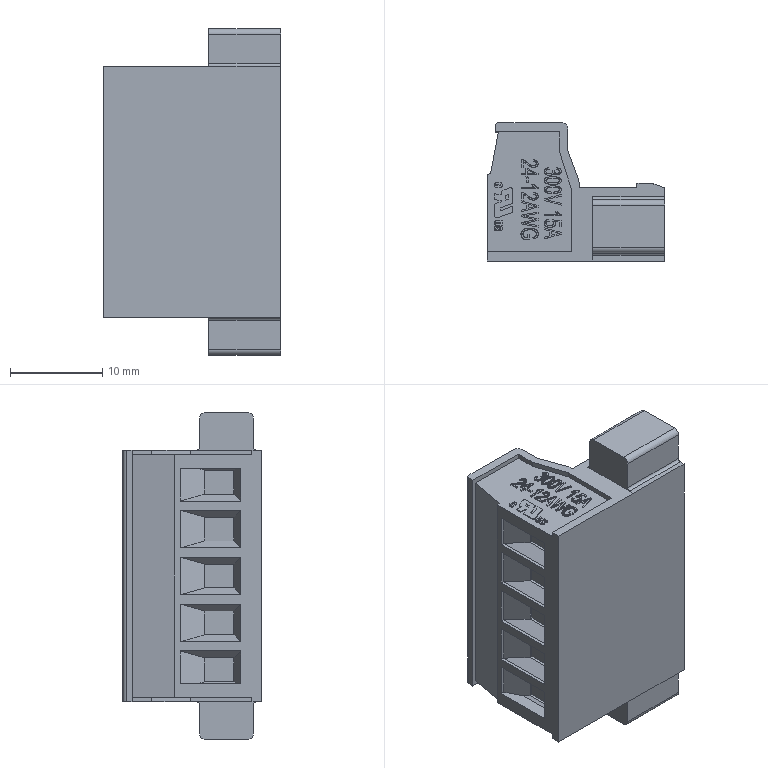Part | NX | features BREP 13 | 13 solids | 3843 faces | volume 4543 mm3 | plane 3503 | cylinder 165 | spline 116 | torus 40 | cone 19 | commonest cylinder face diameters 3.2 x40 3.6 x36 3.9 x10 4 x10 0.677 x6 6 x5